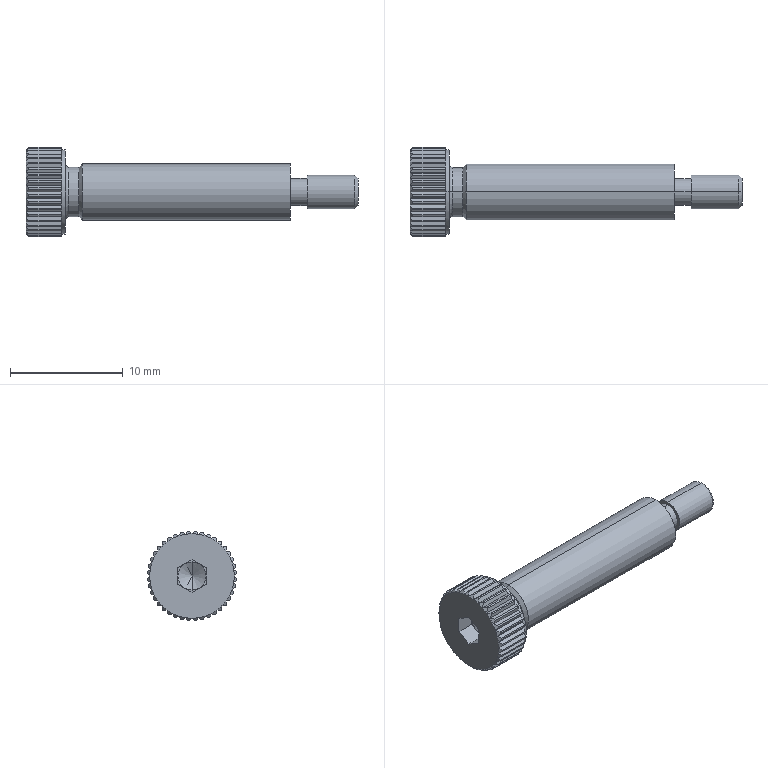Part | STEP file | 001-004-TBH02_d5_L20 | 1 solid | 235 faces | box 29.5 x 7.985 x 7.985 mm | volume 581.04 mm3 | plane 137 | cylinder 50 | cone 46 | torus 2 | commonest cylinder face diameters 8 x40 2.4 x2 3 x2 4.4 x2 5 x2 7.5 x2